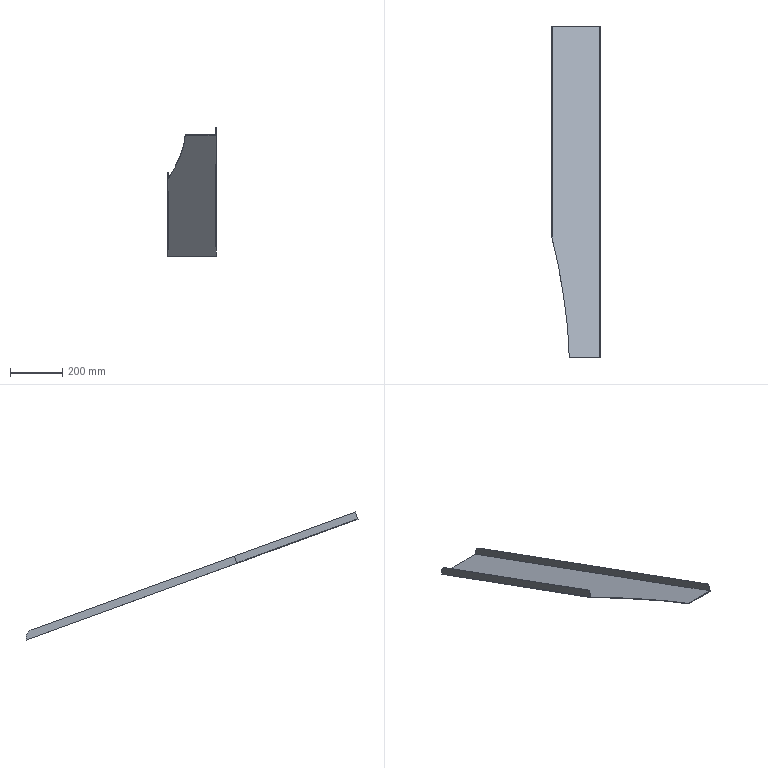Part | NX | features solid 2 | 1 solid | 15 faces | box 185.377 x 1270 x 489.666 mm | volume 582947 mm3 | plane 11 | spline 2 | cylinder 2 | commonest cylinder face diameters 60 x2
STEP:
#1=CARTESIAN_POINT('',(-110.,1180.,-569.375));
#2=VERTEX_POINT('',#1);
#3=CARTESIAN_POINT('',(-110.,-87.894,-107.899));
#4=VERTEX_POINT('',#3);
#5=CARTESIAN_POINT('',(-110.,-155.,-83.474));
#6=DIRECTION('',(0.,-0.9397,0.342));
#7=VECTOR('',#6,1000.);
#8=LINE('',#5,#7);
#9=EDGE_CURVE('',#2,#4,#8,.T.);
#10=ORIENTED_EDGE('',*,*,#9,.F.);
#11=CARTESIAN_POINT('',(-110.,1162.07,-530.923));
#12=VERTEX_POINT('',#11);
#13=CARTESIAN_POINT('',(-110.,1151.809,-559.114));
#14=DIRECTION('',(-1.,0.,0.));
#15=DIRECTION('',(0.,0.,1.));
#16=AXIS2_PLACEMENT_3D('',#13,#14,#15);
#17=CIRCLE('',#16,30.);
#18=EDGE_CURVE('',#2,#12,#17,.F.);
#19=ORIENTED_EDGE('',*,*,#18,.T.);
#20=CARTESIAN_POINT('',(-110.,-77.633,-79.708));
#21=VERTEX_POINT('',#20);
#22=CARTESIAN_POINT('',(-110.,1190.261,-541.184));
#23=DIRECTION('',(0.,-0.9397,0.342));
#24=VECTOR('',#23,1000.);
#25=LINE('',#22,#24);
#26=EDGE_CURVE('',#12,#21,#25,.T.);
#27=ORIENTED_EDGE('',*,*,#26,.T.);
#28=CARTESIAN_POINT('',(-110.,-87.21,-106.02));
#29=DIRECTION('',(0.,-0.342,-0.9397));
#30=VECTOR('',#29,1000.);
#31=LINE('',#28,#30);
#32=EDGE_CURVE('',#21,#4,#31,.T.);
#33=ORIENTED_EDGE('',*,*,#32,.T.);
#34=EDGE_LOOP('',(#10,#19,#27,#33));
#35=FACE_BOUND('',#34,.T.);
#36=CARTESIAN_POINT('',(-110.,-154.316,-81.595));
#37=DIRECTION('',(1.,0.,0.));
#38=DIRECTION('',(0.,0.,-1.));
#39=AXIS2_PLACEMENT_3D('',#36,#37,#38);
#40=PLANE('',#39);
#41=ADVANCED_FACE('',(#35),#40,.T.);
#42=CARTESIAN_POINT('',(-112.,1180.,-569.375));
#43=VERTEX_POINT('',#42);
#44=CARTESIAN_POINT('',(-112.,1180.,-567.246));
#45=VERTEX_POINT('',#44);
#46=CARTESIAN_POINT('',(-112.,1180.,-730.));
#47=DIRECTION('',(0.,0.,-1.));
#48=VECTOR('',#47,1000.);
#49=LINE('',#46,#48);
#50=EDGE_CURVE('',#43,#45,#49,.F.);
#51=ORIENTED_EDGE('',*,*,#50,.F.);
#52=CARTESIAN_POINT('',(-293.377,1180.,-569.375));
#53=VERTEX_POINT('',#52);
#54=CARTESIAN_POINT('',(-625.,1180.,-569.375));
#55=DIRECTION('',(-1.,0.,0.));
#56=VECTOR('',#55,1000.);
#57=LINE('',#54,#56);
#58=EDGE_CURVE('',#53,#43,#57,.F.);
#59=ORIENTED_EDGE('',*,*,#58,.F.);
#60=CARTESIAN_POINT('',(-293.377,1180.,-567.246));
#61=VERTEX_POINT('',#60);
#62=CARTESIAN_POINT('',(-293.377,1180.,-730.));
#63=DIRECTION('',(0.,0.,1.));
#64=VECTOR('',#63,1000.);
#65=LINE('',#62,#64);
#66=EDGE_CURVE('',#61,#53,#65,.F.);
#67=ORIENTED_EDGE('',*,*,#66,.F.);
#68=CARTESIAN_POINT('',(-625.,1180.,-567.246));
#69=DIRECTION('',(-1.,0.,0.));
#70=VECTOR('',#69,1000.);
#71=LINE('',#68,#70);
#72=EDGE_CURVE('',#61,#45,#71,.F.);
#73=ORIENTED_EDGE('',*,*,#72,.T.);
#74=EDGE_LOOP('',(#51,#59,#67,#73));
#75=FACE_BOUND('',#74,.T.);
#76=CARTESIAN_POINT('',(-625.,1180.,-730.));
#77=DIRECTION('',(0.,-1.,0.));
#78=DIRECTION('',(1.,0.,0.));
#79=AXIS2_PLACEMENT_3D('',#76,#77,#78);
#80=PLANE('',#79);
#81=ADVANCED_FACE('',(#75),#80,.F.);
#82=CARTESIAN_POINT('',(-295.377,1162.07,-530.923));
#83=VERTEX_POINT('',#82);
#84=CARTESIAN_POINT('',(-295.377,1180.,-569.375));
#85=VERTEX_POINT('',#84);
#86=CARTESIAN_POINT('',(-295.377,1151.809,-559.114));
#87=DIRECTION('',(1.,0.,0.));
#88=DIRECTION('',(0.,0.,-1.));
#89=AXIS2_PLACEMENT_3D('',#86,#87,#88);
#90=CIRCLE('',#89,30.);
#91=EDGE_CURVE('',#83,#85,#90,.F.);
#92=ORIENTED_EDGE('',*,*,#91,.T.);
#93=CARTESIAN_POINT('',(-295.377,375.,-276.379));
#94=VERTEX_POINT('',#93);
#95=CARTESIAN_POINT('',(-295.377,-155.,-83.474));
#96=DIRECTION('',(0.,-0.9397,0.342));
#97=VECTOR('',#96,1000.);
#98=LINE('',#95,#97);
#99=EDGE_CURVE('',#94,#85,#98,.F.);
#100=ORIENTED_EDGE('',*,*,#99,.F.);
#101=CARTESIAN_POINT('',(-295.377,375.684,-274.499));
#102=VERTEX_POINT('',#101);
#103=CARTESIAN_POINT('',(-295.377,375.,-276.379));
#104=CARTESIAN_POINT('',(-295.377,375.228,-275.752));
#105=CARTESIAN_POINT('',(-295.377,375.456,-275.126));
#106=CARTESIAN_POINT('',(-295.377,375.684,-274.499));
#107=B_SPLINE_CURVE_WITH_KNOTS('',3,(#103,#104,#105,#106),.UNSPECIFIED.,.F.,.F.,(4,4),(0.,1.),.UNSPECIFIED.);
#108=EDGE_CURVE('',#102,#94,#107,.F.);
#109=ORIENTED_EDGE('',*,*,#108,.F.);
#110=CARTESIAN_POINT('',(-295.377,385.261,-248.188));
#111=VERTEX_POINT('',#110);
#112=CARTESIAN_POINT('',(-295.377,375.,-276.379));
#113=DIRECTION('',(0.,0.342,0.9397));
#114=VECTOR('',#113,1000.);
#115=LINE('',#112,#114);
#116=EDGE_CURVE('',#102,#111,#115,.T.);
#117=ORIENTED_EDGE('',*,*,#116,.T.);
#118=CARTESIAN_POINT('',(-295.377,385.261,-248.188));
#119=DIRECTION('',(0.,0.9397,-0.342));
#120=VECTOR('',#119,1000.);
#121=LINE('',#118,#120);
#122=EDGE_CURVE('',#111,#83,#121,.T.);
#123=ORIENTED_EDGE('',*,*,#122,.T.);
#124=EDGE_LOOP('',(#92,#100,#109,#117,#123));
#125=FACE_BOUND('',#124,.T.);
#126=CARTESIAN_POINT('',(-295.377,-154.316,-81.595));
#127=DIRECTION('',(-1.,0.,0.));
#128=DIRECTION('',(0.,0.,1.));
#129=AXIS2_PLACEMENT_3D('',#126,#127,#128);
#130=PLANE('',#129);
#131=ADVANCED_FACE('',(#125),#130,.T.);
#132=CARTESIAN_POINT('',(-234.833,27.777,-150.));
#133=VERTEX_POINT('',#132);
#134=CARTESIAN_POINT('',(-295.377,375.,-276.379));
#135=CARTESIAN_POINT('',(-294.522,371.544,-275.121));
#136=CARTESIAN_POINT('',(-293.394,366.986,-273.462));
#137=CARTESIAN_POINT('',(-292.2,362.161,-271.706));
#138=CARTESIAN_POINT('',(-291.46,359.167,-270.616));
#139=CARTESIAN_POINT('',(-290.874,356.799,-269.754));
#140=CARTESIAN_POINT('',(-290.515,355.348,-269.226));
#141=CARTESIAN_POINT('',(-290.305,354.499,-268.917));
#142=CARTESIAN_POINT('',(-290.207,354.1,-268.772));
#143=CARTESIAN_POINT('',(-290.147,353.857,-268.683));
#144=CARTESIAN_POINT('',(-290.112,353.717,-268.632));
#145=CARTESIAN_POINT('',(-290.089,353.624,-268.598));
#146=CARTESIAN_POINT('',(-290.082,353.594,-268.588));
#147=CARTESIAN_POINT('',(-290.071,353.553,-268.573));
#148=CARTESIAN_POINT('',(-290.085,353.606,-268.592));
#149=CARTESIAN_POINT('',(-290.021,353.351,-268.499));
#150=CARTESIAN_POINT('',(-289.964,353.118,-268.414));
#151=CARTESIAN_POINT('',(-289.851,352.663,-268.249));
#152=CARTESIAN_POINT('',(-289.698,352.041,-268.022));
#153=CARTESIAN_POINT('',(-289.513,351.29,-267.749));
#154=CARTESIAN_POINT('',(-289.269,350.301,-267.389));
#155=CARTESIAN_POINT('',(-288.968,349.077,-266.943));
#156=CARTESIAN_POINT('',(-288.495,347.15,-266.242));
#157=CARTESIAN_POINT('',(-287.919,344.799,-265.386));
#158=CARTESIAN_POINT('',(-287.031,341.162,-264.063));
#159=CARTESIAN_POINT('',(-286.193,337.702,-262.803));
#160=CARTESIAN_POINT('',(-285.507,334.856,-261.767));
#161=CARTESIAN_POINT('',(-285.121,333.246,-261.182));
#162=CARTESIAN_POINT('',(-284.857,332.144,-260.78));
#163=CARTESIAN_POINT('',(-284.526,330.753,-260.274));
#164=CARTESIAN_POINT('',(-284.109,328.997,-259.635));
#165=CARTESIAN_POINT('',(-283.371,325.875,-258.499));
#166=CARTESIAN_POINT('',(-282.331,321.43,-256.881));
#167=CARTESIAN_POINT('',(-281.095,316.07,-254.93));
#168=CARTESIAN_POINT('',(-279.466,308.904,-252.322));
#169=CARTESIAN_POINT('',(-277.468,299.924,-249.053));
#170=CARTESIAN_POINT('',(-275.11,289.007,-245.08));
#171=CARTESIAN_POINT('',(-272.869,278.318,-241.189));
#172=CARTESIAN_POINT('',(-270.673,267.536,-237.265));
#173=CARTESIAN_POINT('',(-268.542,256.746,-233.338));
#174=CARTESIAN_POINT('',(-266.471,245.925,-229.399));
#175=CARTESIAN_POINT('',(-264.796,236.888,-226.11));
#176=CARTESIAN_POINT('',(-263.487,229.645,-223.474));
#177=CARTESIAN_POINT('',(-262.52,224.206,-221.494));
#178=CARTESIAN_POINT('',(-261.569,218.761,-219.512));
#179=CARTESIAN_POINT('',(-260.788,214.218,-217.859));
#180=CARTESIAN_POINT('',(-260.172,210.581,-216.535));
#181=CARTESIAN_POINT('',(-259.789,208.306,-215.707));
#182=CARTESIAN_POINT('',(-259.486,206.486,-215.044));
#183=CARTESIAN_POINT('',(-259.258,205.118,-214.547));
#184=CARTESIAN_POINT('',(-259.071,203.985,-214.134));
#185=CARTESIAN_POINT('',(-258.938,203.177,-213.84));
#186=CARTESIAN_POINT('',(-258.866,202.739,-213.681));
#187=CARTESIAN_POINT('',(-258.801,202.344,-213.537));
#188=CARTESIAN_POINT('',(-258.777,202.201,-213.485));
#189=CARTESIAN_POINT('',(-258.731,201.919,-213.382));
#190=CARTESIAN_POINT('',(-258.655,201.457,-213.214));
#191=CARTESIAN_POINT('',(-258.541,200.755,-212.959));
#192=CARTESIAN_POINT('',(-258.399,199.884,-212.642));
#193=CARTESIAN_POINT('',(-258.203,198.672,-212.2));
#194=CARTESIAN_POINT('',(-257.944,197.067,-211.616));
#195=CARTESIAN_POINT('',(-257.5,194.306,-210.612));
#196=CARTESIAN_POINT('',(-256.893,190.493,-209.224));
#197=CARTESIAN_POINT('',(-256.077,185.337,-207.347));
#198=CARTESIAN_POINT('',(-255.175,179.603,-205.26));
#199=CARTESIAN_POINT('',(-254.351,174.341,-203.345));
#200=CARTESIAN_POINT('',(-253.65,169.842,-201.707));
#201=CARTESIAN_POINT('',(-253.101,166.32,-200.425));
#202=CARTESIAN_POINT('',(-252.628,163.276,-199.317));
#203=CARTESIAN_POINT('',(-252.284,161.059,-198.51));
#204=CARTESIAN_POINT('',(-252.09,159.809,-198.056));
#205=CARTESIAN_POINT('',(-251.928,158.763,-197.675));
#206=CARTESIAN_POINT('',(-251.823,158.091,-197.43));
#207=CARTESIAN_POINT('',(-251.665,157.071,-197.059));
#208=CARTESIAN_POINT('',(-251.4,155.363,-196.437));
#209=CARTESIAN_POINT('',(-251.023,152.936,-195.554));
#210=CARTESIAN_POINT('',(-250.584,150.108,-194.525));
#211=CARTESIAN_POINT('',(-250.155,147.348,-193.52));
#212=CARTESIAN_POINT('',(-249.736,144.661,-192.542));
#213=CARTESIAN_POINT('',(-249.396,142.48,-191.748));
#214=CARTESIAN_POINT('',(-249.13,140.771,-191.126));
#215=CARTESIAN_POINT('',(-248.933,139.509,-190.667));
#216=CARTESIAN_POINT('',(-248.77,138.465,-190.287));
#217=CARTESIAN_POINT('',(-248.659,137.756,-190.029));
#218=CARTESIAN_POINT('',(-248.593,137.331,-189.874));
#219=CARTESIAN_POINT('',(-248.553,137.076,-189.781));
#220=CARTESIAN_POINT('',(-248.476,136.582,-189.602));
#221=CARTESIAN_POINT('',(-248.387,136.012,-189.394));
#222=CARTESIAN_POINT('',(-248.227,134.988,-189.021));
#223=CARTESIAN_POINT('',(-248.007,133.577,-188.508));
#224=CARTESIAN_POINT('',(-247.75,131.927,-187.907));
#225=CARTESIAN_POINT('',(-247.419,129.799,-187.133));
#226=CARTESIAN_POINT('',(-247.027,127.269,-186.212));
#227=CARTESIAN_POINT('',(-246.445,123.497,-184.839));
#228=CARTESIAN_POINT('',(-245.933,120.148,-183.62));
#229=CARTESIAN_POINT('',(-245.542,117.565,-182.68));
#230=CARTESIAN_POINT('',(-245.364,116.387,-182.251));
#231=CARTESIAN_POINT('',(-245.262,115.705,-182.003));
#232=CARTESIAN_POINT('',(-245.202,115.303,-181.857));
#233=CARTESIAN_POINT('',(-245.089,114.544,-181.58));
#234=CARTESIAN_POINT('',(-244.957,113.656,-181.257));
#235=CARTESIAN_POINT('',(-244.787,112.504,-180.838));
#236=CARTESIAN_POINT('',(-244.587,111.14,-180.341));
#237=CARTESIAN_POINT('',(-244.32,109.315,-179.677));
#238=CARTESIAN_POINT('',(-243.991,107.035,-178.848));
#239=CARTESIAN_POINT('',(-243.471,103.388,-177.52));
#240=CARTESIAN_POINT('',(-242.834,98.829,-175.861));
#241=CARTESIAN_POINT('',(-242.091,93.359,-173.87));
#242=CARTESIAN_POINT('',(-241.369,87.889,-171.879));
#243=CARTESIAN_POINT('',(-240.435,80.598,-169.225));
#244=CARTESIAN_POINT('',(-238.874,67.841,-164.582));
#245=CARTESIAN_POINT('',(-236.855,49.624,-157.951));
#246=CARTESIAN_POINT('',(-235.465,35.058,-152.65));
#247=CARTESIAN_POINT('',(-234.826,27.777,-150.));
#248=B_SPLINE_CURVE_WITH_KNOTS('',3,(#134,#135,#136,#137,#138,#139,#140,#141,#142,#143,#144,#145,#146,#147,#148,#149,#150,#151,#152,#153,#154,#155,#156,#157,#158,#159,#160,#161,#162,#163,#164,#165,#166,#167,#168,#169,#170,#171,#172,#173,#174,#175,#176,#177,#178,#179,#180,#181,#182,#183,#184,#185,#186,#187,#188,#189,#190,#191,#192,#193,#194,#195,#196,#197,#198,#199,#200,#201,#202,#203,#204,#205,#206,#207,#208,#209,#210,#211,#212,#213,#214,#215,#216,#217,#218,#219,#220,#221,#222,#223,#224,#225,#226,#227,#228,#229,#230,#231,#232,#233,#234,#235,#236,#237,#238,#239,#240,#241,#242,#243,#244,#245,#246,#247),.UNSPECIFIED.,.F.,.F.,(4,1,1,1,1,1,1,1,1,1,1,1,1,1,1,1,1,1,1,1,1,1,1,1,1,1,1,1,1,1,1,1,1,1,1,1,1,1,1,1,1,1,1,1,1,1,1,1,1,1,1,1,1,1,1,1,1,1,1,1,1,1,1,1,1,1,1,1,1,1,1,1,1,1,1,1,1,1,1,1,1,1,1,1,1,1,1,1,1,1,1,1,1,1,1,1,1,1,1,1,1,1,1,1,1,1,1,1,1,1,1,4),(0.,0.01562,0.02344,0.03125,0.03906,0.04688,0.05078,0.05469,0.05664,0.05859,0.06055,0.06152,0.06201,0.0625,0.06299,0.06348,0.06445,0.06641,0.06836,0.07031,0.07422,0.07812,0.08594,0.09375,0.1094,0.1172,0.1211,0.125,0.1289,0.1328,0.1406,0.1562,0.1719,0.1875,0.2188,0.25,0.2812,0.3125,0.3438,0.375,0.4062,0.4219,0.4375,0.4531,0.4688,0.4766,0.4844,0.4883,0.4922,0.4961,0.498,0.499,0.5,0.501,0.502,0.5039,0.5078,0.5117,0.5156,0.5234,0.5312,0.5469,0.5625,0.5781,0.5938,0.6016,0.6094,0.6172,0.6211,0.623,0.625,0.627,0.6289,0.6328,0.6406,0.6484,0.6562,0.6641,0.6719,0.6758,0.6797,0.6836,0.6855,0.6865,0.6875,0.6885,0.6895,0.6914,0.6953,0.6992,0.7031,0.7109,0.7188,0.7344,0.7422,0.7461,0.748,0.75,0.752,0.7539,0.7578,0.7617,0.7656,0.7734,0.7812,0.7969,0.8125,0.8281,0.8438,0.875,0.9375,1.),.UNSPECIFIED.);
#249=EDGE_CURVE('',#94,#133,#248,.T.);
#250=ORIENTED_EDGE('',*,*,#249,.T.);
#251=CARTESIAN_POINT('',(-234.833,28.461,-148.121));
#252=VERTEX_POINT('',#251);
#253=CARTESIAN_POINT('',(-234.826,27.778,-150.));
#254=CARTESIAN_POINT('',(-234.826,28.006,-149.374));
#255=CARTESIAN_POINT('',(-234.826,28.234,-148.747));
#256=CARTESIAN_POINT('',(-234.826,28.462,-148.121));
#257=B_SPLINE_CURVE_WITH_KNOTS('',3,(#253,#254,#255,#256),.UNSPECIFIED.,.F.,.F.,(4,4),(0.,1.),.UNSPECIFIED.);
#258=EDGE_CURVE('',#252,#133,#257,.F.);
#259=ORIENTED_EDGE('',*,*,#258,.F.);
#260=CARTESIAN_POINT('',(-295.377,375.684,-274.499));
#261=CARTESIAN_POINT('',(-294.522,372.228,-273.241));
#262=CARTESIAN_POINT('',(-293.394,367.67,-271.583));
#263=CARTESIAN_POINT('',(-292.2,362.845,-269.826));
#264=CARTESIAN_POINT('',(-291.46,359.851,-268.737));
#265=CARTESIAN_POINT('',(-290.874,357.483,-267.875));
#266=CARTESIAN_POINT('',(-290.515,356.032,-267.346));
#267=CARTESIAN_POINT('',(-290.305,355.183,-267.038));
#268=CARTESIAN_POINT('',(-290.207,354.784,-266.892));
#269=CARTESIAN_POINT('',(-290.147,354.541,-266.804));
#270=CARTESIAN_POINT('',(-290.112,354.401,-266.753));
#271=CARTESIAN_POINT('',(-290.089,354.308,-266.719));
#272=CARTESIAN_POINT('',(-290.082,354.278,-266.708));
#273=CARTESIAN_POINT('',(-290.071,354.237,-266.693));
#274=CARTESIAN_POINT('',(-290.085,354.29,-266.713));
#275=CARTESIAN_POINT('',(-290.021,354.035,-266.62));
#276=CARTESIAN_POINT('',(-289.964,353.802,-266.535));
#277=CARTESIAN_POINT('',(-289.851,353.347,-266.369));
#278=CARTESIAN_POINT('',(-289.698,352.725,-266.143));
#279=CARTESIAN_POINT('',(-289.513,351.975,-265.87));
#280=CARTESIAN_POINT('',(-289.269,350.985,-265.51));
#281=CARTESIAN_POINT('',(-288.968,349.761,-265.064));
#282=CARTESIAN_POINT('',(-288.495,347.834,-264.363));
#283=CARTESIAN_POINT('',(-287.919,345.483,-263.507));
#284=CARTESIAN_POINT('',(-287.031,341.846,-262.183));
#285=CARTESIAN_POINT('',(-286.193,338.386,-260.924));
#286=CARTESIAN_POINT('',(-285.507,335.54,-259.888));
#287=CARTESIAN_POINT('',(-285.121,333.93,-259.302));
#288=CARTESIAN_POINT('',(-284.857,332.828,-258.901));
#289=CARTESIAN_POINT('',(-284.526,331.437,-258.395));
#290=CARTESIAN_POINT('',(-284.109,329.682,-257.756));
#291=CARTESIAN_POINT('',(-283.371,326.559,-256.619));
#292=CARTESIAN_POINT('',(-282.331,322.114,-255.001));
#293=CARTESIAN_POINT('',(-281.095,316.754,-253.05));
#294=CARTESIAN_POINT('',(-279.466,309.588,-250.442));
#295=CARTESIAN_POINT('',(-277.468,300.608,-247.174));
#296=CARTESIAN_POINT('',(-275.11,289.691,-243.201));
#297=CARTESIAN_POINT('',(-272.869,279.002,-239.31));
#298=CARTESIAN_POINT('',(-270.673,268.22,-235.386));
#299=CARTESIAN_POINT('',(-268.542,257.43,-231.458));
#300=CARTESIAN_POINT('',(-266.471,246.609,-227.52));
#301=CARTESIAN_POINT('',(-264.796,237.572,-224.231));
#302=CARTESIAN_POINT('',(-263.487,230.329,-221.594));
#303=CARTESIAN_POINT('',(-262.52,224.89,-219.615));
#304=CARTESIAN_POINT('',(-261.569,219.445,-217.633));
#305=CARTESIAN_POINT('',(-260.788,214.902,-215.979));
#306=CARTESIAN_POINT('',(-260.172,211.265,-214.656));
#307=CARTESIAN_POINT('',(-259.789,208.99,-213.827));
#308=CARTESIAN_POINT('',(-259.486,207.17,-213.165));
#309=CARTESIAN_POINT('',(-259.258,205.802,-212.667));
#310=CARTESIAN_POINT('',(-259.071,204.669,-212.255));
#311=CARTESIAN_POINT('',(-258.938,203.861,-211.961));
#312=CARTESIAN_POINT('',(-258.866,203.423,-211.801));
#313=CARTESIAN_POINT('',(-258.801,203.028,-211.658));
#314=CARTESIAN_POINT('',(-258.777,202.885,-211.606));
#315=CARTESIAN_POINT('',(-258.731,202.603,-211.503));
#316=CARTESIAN_POINT('',(-258.655,202.141,-211.335));
#317=CARTESIAN_POINT('',(-258.541,201.439,-211.079));
#318=CARTESIAN_POINT('',(-258.399,200.568,-210.762));
#319=CARTESIAN_POINT('',(-258.203,199.356,-210.321));
#320=CARTESIAN_POINT('',(-257.944,197.751,-209.737));
#321=CARTESIAN_POINT('',(-257.5,194.99,-208.732));
#322=CARTESIAN_POINT('',(-256.893,191.177,-207.344));
#323=CARTESIAN_POINT('',(-256.077,186.022,-205.468));
#324=CARTESIAN_POINT('',(-255.175,180.287,-203.381));
#325=CARTESIAN_POINT('',(-254.351,175.025,-201.465));
#326=CARTESIAN_POINT('',(-253.65,170.526,-199.828));
#327=CARTESIAN_POINT('',(-253.101,167.004,-198.546));
#328=CARTESIAN_POINT('',(-252.628,163.96,-197.438));
#329=CARTESIAN_POINT('',(-252.284,161.743,-196.631));
#330=CARTESIAN_POINT('',(-252.09,160.493,-196.176));
#331=CARTESIAN_POINT('',(-251.928,159.447,-195.795));
#332=CARTESIAN_POINT('',(-251.823,158.775,-195.551));
#333=CARTESIAN_POINT('',(-251.665,157.755,-195.18));
#334=CARTESIAN_POINT('',(-251.4,156.047,-194.558));
#335=CARTESIAN_POINT('',(-251.023,153.62,-193.675));
#336=CARTESIAN_POINT('',(-250.584,150.793,-192.645));
#337=CARTESIAN_POINT('',(-250.155,148.033,-191.641));
#338=CARTESIAN_POINT('',(-249.736,145.345,-190.663));
#339=CARTESIAN_POINT('',(-249.396,143.164,-189.869));
#340=CARTESIAN_POINT('',(-249.13,141.455,-189.247));
#341=CARTESIAN_POINT('',(-248.933,140.193,-188.788));
#342=CARTESIAN_POINT('',(-248.77,139.149,-188.407));
#343=CARTESIAN_POINT('',(-248.659,138.44,-188.15));
#344=CARTESIAN_POINT('',(-248.593,138.015,-187.995));
#345=CARTESIAN_POINT('',(-248.553,137.76,-187.902));
#346=CARTESIAN_POINT('',(-248.476,137.266,-187.722));
#347=CARTESIAN_POINT('',(-248.387,136.697,-187.515));
#348=CARTESIAN_POINT('',(-248.227,135.672,-187.142));
#349=CARTESIAN_POINT('',(-248.007,134.261,-186.628));
#350=CARTESIAN_POINT('',(-247.75,132.611,-186.028));
#351=CARTESIAN_POINT('',(-247.419,130.483,-185.253));
#352=CARTESIAN_POINT('',(-247.027,127.953,-184.332));
#353=CARTESIAN_POINT('',(-246.445,124.181,-182.96));
#354=CARTESIAN_POINT('',(-245.933,120.832,-181.741));
#355=CARTESIAN_POINT('',(-245.542,118.249,-180.801));
#356=CARTESIAN_POINT('',(-245.364,117.071,-180.372));
#357=CARTESIAN_POINT('',(-245.262,116.389,-180.123));
#358=CARTESIAN_POINT('',(-245.202,115.987,-179.977));
#359=CARTESIAN_POINT('',(-245.089,115.228,-179.701));
#360=CARTESIAN_POINT('',(-244.957,114.34,-179.378));
#361=CARTESIAN_POINT('',(-244.787,113.188,-178.959));
#362=CARTESIAN_POINT('',(-244.587,111.824,-178.462));
#363=CARTESIAN_POINT('',(-244.32,109.999,-177.798));
#364=CARTESIAN_POINT('',(-243.991,107.719,-176.968));
#365=CARTESIAN_POINT('',(-243.471,104.072,-175.64));
#366=CARTESIAN_POINT('',(-242.834,99.513,-173.981));
#367=CARTESIAN_POINT('',(-242.091,94.043,-171.99));
#368=CARTESIAN_POINT('',(-241.369,88.573,-170.));
#369=CARTESIAN_POINT('',(-240.435,81.282,-167.346));
#370=CARTESIAN_POINT('',(-238.874,68.525,-162.702));
#371=CARTESIAN_POINT('',(-236.855,50.308,-156.072));
#372=CARTESIAN_POINT('',(-235.465,35.742,-150.771));
#373=CARTESIAN_POINT('',(-234.826,28.462,-148.121));
#374=B_SPLINE_CURVE_WITH_KNOTS('',3,(#260,#261,#262,#263,#264,#265,#266,#267,#268,#269,#270,#271,#272,#273,#274,#275,#276,#277,#278,#279,#280,#281,#282,#283,#284,#285,#286,#287,#288,#289,#290,#291,#292,#293,#294,#295,#296,#297,#298,#299,#300,#301,#302,#303,#304,#305,#306,#307,#308,#309,#310,#311,#312,#313,#314,#315,#316,#317,#318,#319,#320,#321,#322,#323,#324,#325,#326,#327,#328,#329,#330,#331,#332,#333,#334,#335,#336,#337,#338,#339,#340,#341,#342,#343,#344,#345,#346,#347,#348,#349,#350,#351,#352,#353,#354,#355,#356,#357,#358,#359,#360,#361,#362,#363,#364,#365,#366,#367,#368,#369,#370,#371,#372,#373),.UNSPECIFIED.,.F.,.F.,(4,1,1,1,1,1,1,1,1,1,1,1,1,1,1,1,1,1,1,1,1,1,1,1,1,1,1,1,1,1,1,1,1,1,1,1,1,1,1,1,1,1,1,1,1,1,1,1,1,1,1,1,1,1,1,1,1,1,1,1,1,1,1,1,1,1,1,1,1,1,1,1,1,1,1,1,1,1,1,1,1,1,1,1,1,1,1,1,1,1,1,1,1,1,1,1,1,1,1,1,1,1,1,1,1,1,1,1,1,1,1,4),(0.,0.01562,0.02344,0.03125,0.03906,0.04688,0.05078,0.05469,0.05664,0.05859,0.06055,0.06152,0.06201,0.0625,0.06299,0.06348,0.06445,0.06641,0.06836,0.07031,0.07422,0.07812,0.08594,0.09375,0.1094,0.1172,0.1211,0.125,0.1289,0.1328,0.1406,0.1562,0.1719,0.1875,0.2188,0.25,0.2812,0.3125,0.3438,0.375,0.4062,0.4219,0.4375,0.4531,0.4688,0.4766,0.4844,0.4883,0.4922,0.4961,0.498,0.499,0.5,0.501,0.502,0.5039,0.5078,0.5117,0.5156,0.5234,0.5312,0.5469,0.5625,0.5781,0.5938,0.6016,0.6094,0.6172,0.6211,0.623,0.625,0.627,0.6289,0.6328,0.6406,0.6484,0.6562,0.6641,0.6719,0.6758,0.6797,0.6836,0.6855,0.6865,0.6875,0.6885,0.6895,0.6914,0.6953,0.6992,0.7031,0.7109,0.7188,0.7344,0.7422,0.7461,0.748,0.75,0.752,0.7539,0.7578,0.7617,0.7656,0.7734,0.7812,0.7969,0.8125,0.8281,0.8438,0.875,0.9375,1.),.UNSPECIFIED.);
#375=EDGE_CURVE('',#102,#252,#374,.T.);
#376=ORIENTED_EDGE('',*,*,#375,.F.);
#377=ORIENTED_EDGE('',*,*,#108,.T.);
#378=EDGE_LOOP('',(#250,#259,#376,#377));
#379=FACE_BOUND('',#378,.T.);
#380=CARTESIAN_POINT('',(-295.377,375.684,-274.499));
#381=CARTESIAN_POINT('',(-295.377,375.,-276.379));
#382=CARTESIAN_POINT('',(-294.522,372.228,-273.241));
#383=CARTESIAN_POINT('',(-294.522,371.544,-275.121));
#384=CARTESIAN_POINT('',(-293.394,367.67,-271.583));
#385=CARTESIAN_POINT('',(-293.394,366.986,-273.462));
#386=CARTESIAN_POINT('',(-292.2,362.845,-269.826));
#387=CARTESIAN_POINT('',(-292.2,362.161,-271.706));
#388=CARTESIAN_POINT('',(-291.46,359.851,-268.737));
#389=CARTESIAN_POINT('',(-291.46,359.167,-270.616));
#390=CARTESIAN_POINT('',(-290.874,357.483,-267.875));
#391=CARTESIAN_POINT('',(-290.874,356.799,-269.754));
#392=CARTESIAN_POINT('',(-290.515,356.032,-267.346));
#393=CARTESIAN_POINT('',(-290.515,355.348,-269.226));
#394=CARTESIAN_POINT('',(-290.305,355.183,-267.038));
#395=CARTESIAN_POINT('',(-290.305,354.499,-268.917));
#396=CARTESIAN_POINT('',(-290.207,354.784,-266.892));
#397=CARTESIAN_POINT('',(-290.207,354.1,-268.772));
#398=CARTESIAN_POINT('',(-290.147,354.541,-266.804));
#399=CARTESIAN_POINT('',(-290.147,353.857,-268.683));
#400=CARTESIAN_POINT('',(-290.112,354.401,-266.753));
#401=CARTESIAN_POINT('',(-290.112,353.717,-268.632));
#402=CARTESIAN_POINT('',(-290.089,354.308,-266.719));
#403=CARTESIAN_POINT('',(-290.089,353.624,-268.598));
#404=CARTESIAN_POINT('',(-290.082,354.278,-266.708));
#405=CARTESIAN_POINT('',(-290.082,353.594,-268.588));
#406=CARTESIAN_POINT('',(-290.071,354.237,-266.693));
#407=CARTESIAN_POINT('',(-290.071,353.553,-268.573));
#408=CARTESIAN_POINT('',(-290.085,354.29,-266.713));
#409=CARTESIAN_POINT('',(-290.085,353.606,-268.592));
#410=CARTESIAN_POINT('',(-290.021,354.035,-266.62));
#411=CARTESIAN_POINT('',(-290.021,353.351,-268.499));
#412=CARTESIAN_POINT('',(-289.964,353.802,-266.535));
#413=CARTESIAN_POINT('',(-289.964,353.118,-268.414));
#414=CARTESIAN_POINT('',(-289.851,353.347,-266.369));
#415=CARTESIAN_POINT('',(-289.851,352.663,-268.249));
#416=CARTESIAN_POINT('',(-289.698,352.725,-266.143));
#417=CARTESIAN_POINT('',(-289.698,352.041,-268.022));
#418=CARTESIAN_POINT('',(-289.513,351.975,-265.87));
#419=CARTESIAN_POINT('',(-289.513,351.29,-267.749));
#420=CARTESIAN_POINT('',(-289.269,350.985,-265.51));
#421=CARTESIAN_POINT('',(-289.269,350.301,-267.389));
#422=CARTESIAN_POINT('',(-288.968,349.761,-265.064));
#423=CARTESIAN_POINT('',(-288.968,349.077,-266.943));
#424=CARTESIAN_POINT('',(-288.495,347.834,-264.363));
#425=CARTESIAN_POINT('',(-288.495,347.15,-266.242));
#426=CARTESIAN_POINT('',(-287.919,345.483,-263.507));
#427=CARTESIAN_POINT('',(-287.919,344.799,-265.386));
#428=CARTESIAN_POINT('',(-287.031,341.846,-262.183));
#429=CARTESIAN_POINT('',(-287.031,341.162,-264.063));
#430=CARTESIAN_POINT('',(-286.193,338.386,-260.924));
#431=CARTESIAN_POINT('',(-286.193,337.702,-262.803));
#432=CARTESIAN_POINT('',(-285.507,335.54,-259.888));
#433=CARTESIAN_POINT('',(-285.507,334.856,-261.767));
#434=CARTESIAN_POINT('',(-285.121,333.93,-259.302));
#435=CARTESIAN_POINT('',(-285.121,333.246,-261.182));
#436=CARTESIAN_POINT('',(-284.857,332.828,-258.901));
#437=CARTESIAN_POINT('',(-284.857,332.144,-260.78));
#438=CARTESIAN_POINT('',(-284.526,331.437,-258.395));
#439=CARTESIAN_POINT('',(-284.526,330.753,-260.274));
#440=CARTESIAN_POINT('',(-284.109,329.682,-257.756));
#441=CARTESIAN_POINT('',(-284.109,328.997,-259.635));
#442=CARTESIAN_POINT('',(-283.371,326.559,-256.619));
#443=CARTESIAN_POINT('',(-283.371,325.875,-258.499));
#444=CARTESIAN_POINT('',(-282.331,322.114,-255.001));
#445=CARTESIAN_POINT('',(-282.331,321.43,-256.881));
#446=CARTESIAN_POINT('',(-281.095,316.754,-253.05));
#447=CARTESIAN_POINT('',(-281.095,316.07,-254.93));
#448=CARTESIAN_POINT('',(-279.466,309.588,-250.442));
#449=CARTESIAN_POINT('',(-279.466,308.904,-252.322));
#450=CARTESIAN_POINT('',(-277.468,300.608,-247.174));
#451=CARTESIAN_POINT('',(-277.468,299.924,-249.053));
#452=CARTESIAN_POINT('',(-275.11,289.691,-243.201));
#453=CARTESIAN_POINT('',(-275.11,289.007,-245.08));
#454=CARTESIAN_POINT('',(-272.869,279.002,-239.31));
#455=CARTESIAN_POINT('',(-272.869,278.318,-241.189));
#456=CARTESIAN_POINT('',(-270.673,268.22,-235.386));
#457=CARTESIAN_POINT('',(-270.673,267.536,-237.265));
#458=CARTESIAN_POINT('',(-268.542,257.43,-231.458));
#459=CARTESIAN_POINT('',(-268.542,256.746,-233.338));
#460=CARTESIAN_POINT('',(-266.471,246.609,-227.52));
#461=CARTESIAN_POINT('',(-266.471,245.925,-229.399));
#462=CARTESIAN_POINT('',(-264.796,237.572,-224.231));
#463=CARTESIAN_POINT('',(-264.796,236.888,-226.11));
#464=CARTESIAN_POINT('',(-263.487,230.329,-221.594));
#465=CARTESIAN_POINT('',(-263.487,229.645,-223.474));
#466=CARTESIAN_POINT('',(-262.52,224.89,-219.615));
#467=CARTESIAN_POINT('',(-262.52,224.206,-221.494));
#468=CARTESIAN_POINT('',(-261.569,219.445,-217.633));
#469=CARTESIAN_POINT('',(-261.569,218.761,-219.512));
#470=CARTESIAN_POINT('',(-260.788,214.902,-215.979));
#471=CARTESIAN_POINT('',(-260.788,214.218,-217.859));
#472=CARTESIAN_POINT('',(-260.172,211.265,-214.656));
#473=CARTESIAN_POINT('',(-260.172,210.581,-216.535));
#474=CARTESIAN_POINT('',(-259.789,208.99,-213.827));
#475=CARTESIAN_POINT('',(-259.789,208.306,-215.707));
#476=CARTESIAN_POINT('',(-259.486,207.17,-213.165));
#477=CARTESIAN_POINT('',(-259.486,206.486,-215.044));
#478=CARTESIAN_POINT('',(-259.258,205.802,-212.667));
#479=CARTESIAN_POINT('',(-259.258,205.118,-214.547));
#480=CARTESIAN_POINT('',(-259.071,204.669,-212.255));
#481=CARTESIAN_POINT('',(-259.071,203.985,-214.134));
#482=CARTESIAN_POINT('',(-258.938,203.861,-211.961));
#483=CARTESIAN_POINT('',(-258.938,203.177,-213.84));
#484=CARTESIAN_POINT('',(-258.866,203.423,-211.801));
#485=CARTESIAN_POINT('',(-258.866,202.739,-213.681));
#486=CARTESIAN_POINT('',(-258.801,203.028,-211.658));
#487=CARTESIAN_POINT('',(-258.801,202.344,-213.537));
#488=CARTESIAN_POINT('',(-258.777,202.885,-211.606));
#489=CARTESIAN_POINT('',(-258.777,202.201,-213.485));
#490=CARTESIAN_POINT('',(-258.731,202.603,-211.503));
#491=CARTESIAN_POINT('',(-258.731,201.919,-213.382));
#492=CARTESIAN_POINT('',(-258.655,202.141,-211.335));
#493=CARTESIAN_POINT('',(-258.655,201.457,-213.214));
#494=CARTESIAN_POINT('',(-258.541,201.439,-211.079));
#495=CARTESIAN_POINT('',(-258.541,200.755,-212.959));
#496=CARTESIAN_POINT('',(-258.399,200.568,-210.762));
#497=CARTESIAN_POINT('',(-258.399,199.884,-212.642));
#498=CARTESIAN_POINT('',(-258.203,199.356,-210.321));
#499=CARTESIAN_POINT('',(-258.203,198.672,-212.2));
#500=CARTESIAN_POINT('',(-257.944,197.751,-209.737));
#501=CARTESIAN_POINT('',(-257.944,197.067,-211.616));
#502=CARTESIAN_POINT('',(-257.5,194.99,-208.732));
#503=CARTESIAN_POINT('',(-257.5,194.306,-210.612));
#504=CARTESIAN_POINT('',(-256.893,191.177,-207.344));
#505=CARTESIAN_POINT('',(-256.893,190.493,-209.224));
#506=CARTESIAN_POINT('',(-256.077,186.022,-205.468));
#507=CARTESIAN_POINT('',(-256.077,185.337,-207.347));
#508=CARTESIAN_POINT('',(-255.175,180.287,-203.381));
#509=CARTESIAN_POINT('',(-255.175,179.603,-205.26));
#510=CARTESIAN_POINT('',(-254.351,175.025,-201.465));
#511=CARTESIAN_POINT('',(-254.351,174.341,-203.345));
#512=CARTESIAN_POINT('',(-253.65,170.526,-199.828));
#513=CARTESIAN_POINT('',(-253.65,169.842,-201.707));
#514=CARTESIAN_POINT('',(-253.101,167.004,-198.546));
#515=CARTESIAN_POINT('',(-253.101,166.32,-200.425));
#516=CARTESIAN_POINT('',(-252.628,163.96,-197.438));
#517=CARTESIAN_POINT('',(-252.628,163.276,-199.317));
#518=CARTESIAN_POINT('',(-252.284,161.743,-196.631));
#519=CARTESIAN_POINT('',(-252.284,161.059,-198.51));
#520=CARTESIAN_POINT('',(-252.09,160.493,-196.176));
#521=CARTESIAN_POINT('',(-252.09,159.809,-198.056));
#522=CARTESIAN_POINT('',(-251.928,159.447,-195.795));
#523=CARTESIAN_POINT('',(-251.928,158.763,-197.675));
#524=CARTESIAN_POINT('',(-251.823,158.775,-195.551));
#525=CARTESIAN_POINT('',(-251.823,158.091,-197.43));
#526=CARTESIAN_POINT('',(-251.665,157.755,-195.18));
#527=CARTESIAN_POINT('',(-251.665,157.071,-197.059));
#528=CARTESIAN_POINT('',(-251.4,156.047,-194.558));
#529=CARTESIAN_POINT('',(-251.4,155.363,-196.437));
#530=CARTESIAN_POINT('',(-251.023,153.62,-193.675));
#531=CARTESIAN_POINT('',(-251.023,152.936,-195.554));
#532=CARTESIAN_POINT('',(-250.584,150.793,-192.645));
#533=CARTESIAN_POINT('',(-250.584,150.108,-194.525));
#534=CARTESIAN_POINT('',(-250.155,148.033,-191.641));
#535=CARTESIAN_POINT('',(-250.155,147.348,-193.52));
#536=CARTESIAN_POINT('',(-249.736,145.345,-190.663));
#537=CARTESIAN_POINT('',(-249.736,144.661,-192.542));
#538=CARTESIAN_POINT('',(-249.396,143.164,-189.869));
#539=CARTESIAN_POINT('',(-249.396,142.48,-191.748));
#540=CARTESIAN_POINT('',(-249.13,141.455,-189.247));
#541=CARTESIAN_POINT('',(-249.13,140.771,-191.126));
#542=CARTESIAN_POINT('',(-248.933,140.193,-188.788));
#543=CARTESIAN_POINT('',(-248.933,139.509,-190.667));
#544=CARTESIAN_POINT('',(-248.77,139.149,-188.407));
#545=CARTESIAN_POINT('',(-248.77,138.465,-190.287));
#546=CARTESIAN_POINT('',(-248.659,138.44,-188.15));
#547=CARTESIAN_POINT('',(-248.659,137.756,-190.029));
#548=CARTESIAN_POINT('',(-248.593,138.015,-187.995));
#549=CARTESIAN_POINT('',(-248.593,137.331,-189.874));
#550=CARTESIAN_POINT('',(-248.553,137.76,-187.902));
#551=CARTESIAN_POINT('',(-248.553,137.076,-189.781));
#552=CARTESIAN_POINT('',(-248.476,137.266,-187.722));
#553=CARTESIAN_POINT('',(-248.476,136.582,-189.602));
#554=CARTESIAN_POINT('',(-248.387,136.697,-187.515));
#555=CARTESIAN_POINT('',(-248.387,136.012,-189.394));
#556=CARTESIAN_POINT('',(-248.227,135.672,-187.142));
#557=CARTESIAN_POINT('',(-248.227,134.988,-189.021));
#558=CARTESIAN_POINT('',(-248.007,134.261,-186.628));
#559=CARTESIAN_POINT('',(-248.007,133.577,-188.508));
#560=CARTESIAN_POINT('',(-247.75,132.611,-186.028));
#561=CARTESIAN_POINT('',(-247.75,131.927,-187.907));
#562=CARTESIAN_POINT('',(-247.419,130.483,-185.253));
#563=CARTESIAN_POINT('',(-247.419,129.799,-187.133));
#564=CARTESIAN_POINT('',(-247.027,127.953,-184.332));
#565=CARTESIAN_POINT('',(-247.027,127.269,-186.212));
#566=CARTESIAN_POINT('',(-246.445,124.181,-182.96));
#567=CARTESIAN_POINT('',(-246.445,123.497,-184.839));
#568=CARTESIAN_POINT('',(-245.933,120.832,-181.741));
#569=CARTESIAN_POINT('',(-245.933,120.148,-183.62));
#570=CARTESIAN_POINT('',(-245.542,118.249,-180.801));
#571=CARTESIAN_POINT('',(-245.542,117.565,-182.68));
#572=CARTESIAN_POINT('',(-245.364,117.071,-180.372));
#573=CARTESIAN_POINT('',(-245.364,116.387,-182.251));
#574=CARTESIAN_POINT('',(-245.262,116.389,-180.123));
#575=CARTESIAN_POINT('',(-245.262,115.705,-182.003));
#576=CARTESIAN_POINT('',(-245.202,115.987,-179.977));
#577=CARTESIAN_POINT('',(-245.202,115.303,-181.857));
#578=CARTESIAN_POINT('',(-245.089,115.228,-179.701));
#579=CARTESIAN_POINT('',(-245.089,114.544,-181.58));
#580=CARTESIAN_POINT('',(-244.957,114.34,-179.378));
#581=CARTESIAN_POINT('',(-244.957,113.656,-181.257));
#582=CARTESIAN_POINT('',(-244.787,113.188,-178.959));
#583=CARTESIAN_POINT('',(-244.787,112.504,-180.838));
#584=CARTESIAN_POINT('',(-244.587,111.824,-178.462));
#585=CARTESIAN_POINT('',(-244.587,111.14,-180.341));
#586=CARTESIAN_POINT('',(-244.32,109.999,-177.798));
#587=CARTESIAN_POINT('',(-244.32,109.315,-179.677));
#588=CARTESIAN_POINT('',(-243.991,107.719,-176.968));
#589=CARTESIAN_POINT('',(-243.991,107.035,-178.848));
#590=CARTESIAN_POINT('',(-243.471,104.072,-175.64));
#591=CARTESIAN_POINT('',(-243.471,103.388,-177.52));
#592=CARTESIAN_POINT('',(-242.834,99.513,-173.981));
#593=CARTESIAN_POINT('',(-242.834,98.829,-175.861));
#594=CARTESIAN_POINT('',(-242.091,94.043,-171.99));
#595=CARTESIAN_POINT('',(-242.091,93.359,-173.87));
#596=CARTESIAN_POINT('',(-241.369,88.573,-170.));
#597=CARTESIAN_POINT('',(-241.369,87.889,-171.879));
#598=CARTESIAN_POINT('',(-240.435,81.282,-167.346));
#599=CARTESIAN_POINT('',(-240.435,80.598,-169.225));
#600=CARTESIAN_POINT('',(-238.874,68.525,-162.702));
#601=CARTESIAN_POINT('',(-238.874,67.841,-164.582));
#602=CARTESIAN_POINT('',(-236.855,50.308,-156.072));
#603=CARTESIAN_POINT('',(-236.855,49.624,-157.951));
#604=CARTESIAN_POINT('',(-235.465,35.742,-150.771));
#605=CARTESIAN_POINT('',(-235.465,35.058,-152.65));
#606=CARTESIAN_POINT('',(-234.826,28.462,-148.121));
#607=CARTESIAN_POINT('',(-234.826,27.777,-150.));
#608=B_SPLINE_SURFACE_WITH_KNOTS('',3,1,((#380,#381),(#382,#383),(#384,#385),(#386,#387),(#388,#389),(#390,#391),(#392,#393),(#394,#395),(#396,#397),(#398,#399),(#400,#401),(#402,#403),(#404,#405),(#406,#407),(#408,#409),(#410,#411),(#412,#413),(#414,#415),(#416,#417),(#418,#419),(#420,#421),(#422,#423),(#424,#425),(#426,#427),(#428,#429),(#430,#431),(#432,#433),(#434,#435),(#436,#437),(#438,#439),(#440,#441),(#442,#443),(#444,#445),(#446,#447),(#448,#449),(#450,#451),(#452,#453),(#454,#455),(#456,#457),(#458,#459),(#460,#461),(#462,#463),(#464,#465),(#466,#467),(#468,#469),(#470,#471),(#472,#473),(#474,#475),(#476,#477),(#478,#479),(#480,#481),(#482,#483),(#484,#485),(#486,#487),(#488,#489),(#490,#491),(#492,#493),(#494,#495),(#496,#497),(#498,#499),(#500,#501),(#502,#503),(#504,#505),(#506,#507),(#508,#509),(#510,#511),(#512,#513),(#514,#515),(#516,#517),(#518,#519),(#520,#521),(#522,#523),(#524,#525),(#526,#527),(#528,#529),(#530,#531),(#532,#533),(#534,#535),(#536,#537),(#538,#539),(#540,#541),(#542,#543),(#544,#545),(#546,#547),(#548,#549),(#550,#551),(#552,#553),(#554,#555),(#556,#557),(#558,#559),(#560,#561),(#562,#563),(#564,#565),(#566,#567),(#568,#569),(#570,#571),(#572,#573),(#574,#575),(#576,#577),(#578,#579),(#580,#581),(#582,#583),(#584,#585),(#586,#587),(#588,#589),(#590,#591),(#592,#593),(#594,#595),(#596,#597),(#598,#599),(#600,#601),(#602,#603),(#604,#605),(#606,#607)),.SURF_OF_LINEAR_EXTRUSION.,.F.,.F.,.F.,(4,1,1,1,1,1,1,1,1,1,1,1,1,1,1,1,1,1,1,1,1,1,1,1,1,1,1,1,1,1,1,1,1,1,1,1,1,1,1,1,1,1,1,1,1,1,1,1,1,1,1,1,1,1,1,1,1,1,1,1,1,1,1,1,1,1,1,1,1,1,1,1,1,1,1,1,1,1,1,1,1,1,1,1,1,1,1,1,1,1,1,1,1,1,1,1,1,1,1,1,1,1,1,1,1,1,1,1,1,1,1,4),(2,2),(0.,0.01562,0.02344,0.03125,0.03906,0.04688,0.05078,0.05469,0.05664,0.05859,0.06055,0.06152,0.06201,0.0625,0.06299,0.06348,0.06445,0.06641,0.06836,0.07031,0.07422,0.07812,0.08594,0.09375,0.1094,0.1172,0.1211,0.125,0.1289,0.1328,0.1406,0.1562,0.1719,0.1875,0.2188,0.25,0.2812,0.3125,0.3438,0.375,0.4062,0.4219,0.4375,0.4531,0.4688,0.4766,0.4844,0.4883,0.4922,0.4961,0.498,0.499,0.5,0.501,0.502,0.5039,0.5078,0.5117,0.5156,0.5234,0.5312,0.5469,0.5625,0.5781,0.5938,0.6016,0.6094,0.6172,0.6211,0.623,0.625,0.627,0.6289,0.6328,0.6406,0.6484,0.6562,0.6641,0.6719,0.6758,0.6797,0.6836,0.6855,0.6865,0.6875,0.6885,0.6895,0.6914,0.6953,0.6992,0.7031,0.7109,0.7188,0.7344,0.7422,0.7461,0.748,0.75,0.752,0.7539,0.7578,0.7617,0.7656,0.7734,0.7812,0.7969,0.8125,0.8281,0.8438,0.875,0.9375,1.),(0.,1.),.UNSPECIFIED.);
#609=ADVANCED_FACE('',(#379),#608,.F.);
#610=CARTESIAN_POINT('',(-228.441,-87.894,-107.899));
#611=VERTEX_POINT('',#610);
#612=CARTESIAN_POINT('',(-234.843,27.777,-150.));
#613=CARTESIAN_POINT('',(-234.001,18.156,-146.498));
#614=CARTESIAN_POINT('',(-232.501,-1.099,-139.49));
#615=CARTESIAN_POINT('',(-230.882,-30.02,-128.964));
#616=CARTESIAN_POINT('',(-229.698,-58.958,-118.431));
#617=CARTESIAN_POINT('',(-228.856,-78.249,-111.41));
#618=CARTESIAN_POINT('',(-228.441,-87.894,-107.899));
#619=B_SPLINE_CURVE_WITH_KNOTS('',3,(#612,#613,#614,#615,#616,#617,#618),.UNSPECIFIED.,.F.,.F.,(4,1,1,1,4),(0.,0.03082,0.06163,0.09245,0.1233),.UNSPECIFIED.);
#620=EDGE_CURVE('',#133,#611,#619,.T.);
#621=ORIENTED_EDGE('',*,*,#620,.T.);
#622=CARTESIAN_POINT('',(-228.441,-87.21,-106.02));
#623=VERTEX_POINT('',#622);
#624=CARTESIAN_POINT('',(-228.441,-87.552,-106.959));
#625=DIRECTION('',(0.,-0.342,-0.9397));
#626=VECTOR('',#625,1000.);
#627=LINE('',#624,#626);
#628=EDGE_CURVE('',#623,#611,#627,.T.);
#629=ORIENTED_EDGE('',*,*,#628,.F.);
#630=CARTESIAN_POINT('',(-234.843,28.461,-148.12));
#631=CARTESIAN_POINT('',(-234.001,18.84,-144.619));
#632=CARTESIAN_POINT('',(-232.501,-0.4153,-137.61));
#633=CARTESIAN_POINT('',(-230.882,-29.336,-127.084));
#634=CARTESIAN_POINT('',(-229.698,-58.274,-116.551));
#635=CARTESIAN_POINT('',(-228.856,-77.565,-109.53));
#636=CARTESIAN_POINT('',(-228.441,-87.21,-106.02));
#637=B_SPLINE_CURVE_WITH_KNOTS('',3,(#630,#631,#632,#633,#634,#635,#636),.UNSPECIFIED.,.F.,.F.,(4,1,1,1,4),(0.,0.03082,0.06163,0.09245,0.1233),.UNSPECIFIED.);
#638=EDGE_CURVE('',#252,#623,#637,.T.);
#639=ORIENTED_EDGE('',*,*,#638,.F.);
#640=ORIENTED_EDGE('',*,*,#258,.T.);
#641=EDGE_LOOP('',(#621,#629,#639,#640));
#642=FACE_BOUND('',#641,.T.);
#643=CARTESIAN_POINT('',(-234.843,28.461,-148.12));
#644=CARTESIAN_POINT('',(-234.843,27.777,-150.));
#645=CARTESIAN_POINT('',(-234.441,23.865,-146.447));
#646=CARTESIAN_POINT('',(-234.441,23.181,-148.327));
#647=CARTESIAN_POINT('',(-233.87,16.965,-143.936));
#648=CARTESIAN_POINT('',(-233.87,16.281,-145.816));
#649=CARTESIAN_POINT('',(-233.175,7.754,-140.584));
#650=CARTESIAN_POINT('',(-233.175,7.07,-142.463));
#651=CARTESIAN_POINT('',(-232.768,1.997,-138.488));
#652=CARTESIAN_POINT('',(-232.768,1.313,-140.368));
#653=CARTESIAN_POINT('',(-232.497,-2.044,-137.018));
#654=CARTESIAN_POINT('',(-232.497,-2.728,-138.897));
#655=CARTESIAN_POINT('',(-232.347,-4.341,-136.182));
#656=CARTESIAN_POINT('',(-232.347,-5.025,-138.061));
#657=CARTESIAN_POINT('',(-232.234,-6.099,-135.542));
#658=CARTESIAN_POINT('',(-232.234,-6.783,-137.421));
#659=CARTESIAN_POINT('',(-232.142,-7.567,-135.007));
#660=CARTESIAN_POINT('',(-232.142,-8.251,-136.887));
#661=CARTESIAN_POINT('',(-232.013,-9.662,-134.245));
#662=CARTESIAN_POINT('',(-232.013,-10.346,-136.124));
#663=CARTESIAN_POINT('',(-231.793,-13.35,-132.902));
#664=CARTESIAN_POINT('',(-231.793,-14.034,-134.782));
#665=CARTESIAN_POINT('',(-231.483,-18.854,-130.899));
#666=CARTESIAN_POINT('',(-231.483,-19.538,-132.779));
#667=CARTESIAN_POINT('',(-231.124,-25.787,-128.376));
#668=CARTESIAN_POINT('',(-231.124,-26.471,-130.255));
#669=CARTESIAN_POINT('',(-230.775,-33.044,-125.734));
#670=CARTESIAN_POINT('',(-230.775,-33.728,-127.614));
#671=CARTESIAN_POINT('',(-230.438,-40.689,-122.952));
#672=CARTESIAN_POINT('',(-230.438,-41.373,-124.831));
#673=CARTESIAN_POINT('',(-230.106,-48.467,-120.121));
#674=CARTESIAN_POINT('',(-230.106,-49.151,-122.));
#675=CARTESIAN_POINT('',(-229.662,-58.791,-116.363));
#676=CARTESIAN_POINT('',(-229.662,-59.475,-118.243));
#677=CARTESIAN_POINT('',(-229.107,-71.712,-111.661));
#678=CARTESIAN_POINT('',(-229.107,-72.396,-113.54));
#679=CARTESIAN_POINT('',(-228.663,-82.044,-107.9));
#680=CARTESIAN_POINT('',(-228.663,-82.728,-109.779));
#681=CARTESIAN_POINT('',(-228.441,-87.21,-106.02));
#682=CARTESIAN_POINT('',(-228.441,-87.894,-107.899));
#683=B_SPLINE_SURFACE_WITH_KNOTS('',3,1,((#643,#644),(#645,#646),(#647,#648),(#649,#650),(#651,#652),(#653,#654),(#655,#656),(#657,#658),(#659,#660),(#661,#662),(#663,#664),(#665,#666),(#667,#668),(#669,#670),(#671,#672),(#673,#674),(#675,#676),(#677,#678),(#679,#680),(#681,#682)),.SURF_OF_LINEAR_EXTRUSION.,.F.,.F.,.F.,(4,1,1,1,1,1,1,1,1,1,1,1,1,1,1,1,1,4),(2,2),(0.000009188,0.2013,0.3019,0.4025,0.4528,0.478,0.5032,0.5283,0.5535,0.6038,0.7044,0.805,0.9057,1.006,1.107,1.208,1.409,1.61),(0.,1.),.UNSPECIFIED.);
#684=ADVANCED_FACE('',(#642),#683,.F.);
#685=CARTESIAN_POINT('',(-70.,-87.894,-107.899));
#686=DIRECTION('',(1.,0.,0.));
#687=VECTOR('',#686,1000.);
#688=LINE('',#685,#687);
#689=EDGE_CURVE('',#611,#4,#688,.T.);
#690=ORIENTED_EDGE('',*,*,#689,.T.);
#691=ORIENTED_EDGE('',*,*,#32,.F.);
#692=CARTESIAN_POINT('',(-112.,-77.633,-79.708));
#693=VERTEX_POINT('',#692);
#694=CARTESIAN_POINT('',(-110.,-77.633,-79.708));
#695=DIRECTION('',(1.,0.,0.));
#696=VECTOR('',#695,1000.);
#697=LINE('',#694,#696);
#698=EDGE_CURVE('',#21,#693,#697,.F.);
#699=ORIENTED_EDGE('',*,*,#698,.T.);
#700=CARTESIAN_POINT('',(-112.,-87.21,-106.02));
#701=VERTEX_POINT('',#700);
#702=CARTESIAN_POINT('',(-112.,-87.894,-107.899));
#703=DIRECTION('',(0.,0.342,0.9397));
#704=VECTOR('',#703,1000.);
#705=LINE('',#702,#704);
#706=EDGE_CURVE('',#701,#693,#705,.T.);
#707=ORIENTED_EDGE('',*,*,#706,.F.);
#708=CARTESIAN_POINT('',(-70.,-87.21,-106.02));
#709=DIRECTION('',(1.,0.,0.));
#710=VECTOR('',#709,1000.);
#711=LINE('',#708,#710);
#712=EDGE_CURVE('',#623,#701,#711,.T.);
#713=ORIENTED_EDGE('',*,*,#712,.F.);
#714=ORIENTED_EDGE('',*,*,#628,.T.);
#715=EDGE_LOOP('',(#690,#691,#699,#707,#713,#714));
#716=FACE_BOUND('',#715,.T.);
#717=CARTESIAN_POINT('',(-70.,-87.21,-106.02));
#718=DIRECTION('',(0.,0.9397,-0.342));
#719=DIRECTION('',(0.,0.342,0.9397));
#720=AXIS2_PLACEMENT_3D('',#717,#718,#719);
#721=PLANE('',#720);
#722=ADVANCED_FACE('',(#716),#721,.F.);
#723=CARTESIAN_POINT('',(-112.,-154.316,-81.595));
#724=DIRECTION('',(0.,-0.9397,0.342));
#725=VECTOR('',#724,1000.);
#726=LINE('',#723,#725);
#727=EDGE_CURVE('',#45,#701,#726,.T.);
#728=ORIENTED_EDGE('',*,*,#727,.F.);
#729=ORIENTED_EDGE('',*,*,#72,.F.);
#730=CARTESIAN_POINT('',(-293.377,375.684,-274.499));
#731=VERTEX_POINT('',#730);
#732=CARTESIAN_POINT('',(-293.377,-154.316,-81.595));
#733=DIRECTION('',(0.,0.9397,-0.342));
#734=VECTOR('',#733,1000.);
#735=LINE('',#732,#734);
#736=EDGE_CURVE('',#731,#61,#735,.T.);
#737=ORIENTED_EDGE('',*,*,#736,.F.);
#738=CARTESIAN_POINT('',(-230.,375.684,-274.499));
#739=DIRECTION('',(-1.,0.,0.));
#740=VECTOR('',#739,1000.);
#741=LINE('',#738,#740);
#742=EDGE_CURVE('',#102,#731,#741,.F.);
#743=ORIENTED_EDGE('',*,*,#742,.F.);
#744=ORIENTED_EDGE('',*,*,#375,.T.);
#745=ORIENTED_EDGE('',*,*,#638,.T.);
#746=ORIENTED_EDGE('',*,*,#712,.T.);
#747=EDGE_LOOP('',(#728,#729,#737,#743,#744,#745,#746));
#748=FACE_BOUND('',#747,.T.);
#749=CARTESIAN_POINT('',(-230.,-154.316,-81.595));
#750=DIRECTION('',(0.,0.342,0.9397));
#751=DIRECTION('',(1.,0.,0.));
#752=AXIS2_PLACEMENT_3D('',#749,#750,#751);
#753=PLANE('',#752);
#754=ADVANCED_FACE('',(#748),#753,.T.);
#755=ORIENTED_EDGE('',*,*,#58,.T.);
#756=CARTESIAN_POINT('',(-110.,1180.,-569.375));
#757=DIRECTION('',(1.,0.,0.));
#758=VECTOR('',#757,1000.);
#759=LINE('',#756,#758);
#760=EDGE_CURVE('',#2,#43,#759,.F.);
#761=ORIENTED_EDGE('',*,*,#760,.F.);
#762=ORIENTED_EDGE('',*,*,#9,.T.);
#763=ORIENTED_EDGE('',*,*,#689,.F.);
#764=ORIENTED_EDGE('',*,*,#620,.F.);
#765=ORIENTED_EDGE('',*,*,#249,.F.);
#766=ORIENTED_EDGE('',*,*,#99,.T.);
#767=CARTESIAN_POINT('',(-625.,1180.,-569.375));
#768=DIRECTION('',(-1.,0.,0.));
#769=VECTOR('',#768,1000.);
#770=LINE('',#767,#769);
#771=EDGE_CURVE('',#85,#53,#770,.F.);
#772=ORIENTED_EDGE('',*,*,#771,.T.);
#773=EDGE_LOOP('',(#755,#761,#762,#763,#764,#765,#766,#772));
#774=FACE_BOUND('',#773,.T.);
#775=CARTESIAN_POINT('',(-230.,-155.,-83.474));
#776=DIRECTION('',(0.,0.342,0.9397));
#777=DIRECTION('',(1.,0.,0.));
#778=AXIS2_PLACEMENT_3D('',#775,#776,#777);
#779=PLANE('',#778);
#780=ADVANCED_FACE('',(#774),#779,.F.);
#781=CARTESIAN_POINT('',(-293.377,385.261,-248.188));
#782=VERTEX_POINT('',#781);
#783=CARTESIAN_POINT('',(-293.377,1162.07,-530.923));
#784=VERTEX_POINT('',#783);
#785=CARTESIAN_POINT('',(-293.377,385.261,-248.188));
#786=DIRECTION('',(0.,0.9397,-0.342));
#787=VECTOR('',#786,1000.);
#788=LINE('',#785,#787);
#789=EDGE_CURVE('',#782,#784,#788,.T.);
#790=ORIENTED_EDGE('',*,*,#789,.T.);
#791=CARTESIAN_POINT('',(-295.377,1162.07,-530.923));
#792=DIRECTION('',(1.,0.,0.));
#793=VECTOR('',#792,1000.);
#794=LINE('',#791,#793);
#795=EDGE_CURVE('',#784,#83,#794,.F.);
#796=ORIENTED_EDGE('',*,*,#795,.T.);
#797=ORIENTED_EDGE('',*,*,#122,.F.);
#798=CARTESIAN_POINT('',(-295.377,385.261,-248.188));
#799=DIRECTION('',(1.,0.,0.));
#800=VECTOR('',#799,1000.);
#801=LINE('',#798,#800);
#802=EDGE_CURVE('',#111,#782,#801,.T.);
#803=ORIENTED_EDGE('',*,*,#802,.T.);
#804=EDGE_LOOP('',(#790,#796,#797,#803));
#805=FACE_BOUND('',#804,.T.);
#806=CARTESIAN_POINT('',(-295.377,385.261,-248.188));
#807=DIRECTION('',(0.,-0.342,-0.9397));
#808=DIRECTION('',(0.,0.9397,-0.342));
#809=AXIS2_PLACEMENT_3D('',#806,#807,#808);
#810=PLANE('',#809);
#811=ADVANCED_FACE('',(#805),#810,.F.);
#812=ORIENTED_EDGE('',*,*,#736,.T.);
#813=ORIENTED_EDGE('',*,*,#66,.T.);
#814=CARTESIAN_POINT('',(-293.377,1151.809,-559.114));
#815=DIRECTION('',(1.,0.,0.));
#816=DIRECTION('',(0.,0.,-1.));
#817=AXIS2_PLACEMENT_3D('',#814,#815,#816);
#818=CIRCLE('',#817,30.);
#819=EDGE_CURVE('',#53,#784,#818,.T.);
#820=ORIENTED_EDGE('',*,*,#819,.T.);
#821=ORIENTED_EDGE('',*,*,#789,.F.);
#822=CARTESIAN_POINT('',(-293.377,375.,-276.379));
#823=DIRECTION('',(0.,0.342,0.9397));
#824=VECTOR('',#823,1000.);
#825=LINE('',#822,#824);
#826=EDGE_CURVE('',#731,#782,#825,.T.);
#827=ORIENTED_EDGE('',*,*,#826,.F.);
#828=EDGE_LOOP('',(#812,#813,#820,#821,#827));
#829=FACE_BOUND('',#828,.T.);
#830=CARTESIAN_POINT('',(-293.377,375.,-276.379));
#831=DIRECTION('',(1.,0.,0.));
#832=DIRECTION('',(0.,0.,-1.));
#833=AXIS2_PLACEMENT_3D('',#830,#831,#832);
#834=PLANE('',#833);
#835=ADVANCED_FACE('',(#829),#834,.T.);
#836=ORIENTED_EDGE('',*,*,#116,.F.);
#837=ORIENTED_EDGE('',*,*,#742,.T.);
#838=ORIENTED_EDGE('',*,*,#826,.T.);
#839=ORIENTED_EDGE('',*,*,#802,.F.);
#840=EDGE_LOOP('',(#836,#837,#838,#839));
#841=FACE_BOUND('',#840,.T.);
#842=CARTESIAN_POINT('',(-295.377,375.,-276.379));
#843=DIRECTION('',(0.,0.9397,-0.342));
#844=DIRECTION('',(0.,0.342,0.9397));
#845=AXIS2_PLACEMENT_3D('',#842,#843,#844);
#846=PLANE('',#845);
#847=ADVANCED_FACE('',(#841),#846,.F.);
#848=ORIENTED_EDGE('',*,*,#91,.F.);
#849=ORIENTED_EDGE('',*,*,#795,.F.);
#850=ORIENTED_EDGE('',*,*,#819,.F.);
#851=ORIENTED_EDGE('',*,*,#771,.F.);
#852=EDGE_LOOP('',(#848,#849,#850,#851));
#853=FACE_BOUND('',#852,.T.);
#854=CARTESIAN_POINT('',(-295.377,1151.809,-559.114));
#855=DIRECTION('',(-1.,0.,0.));
#856=DIRECTION('',(0.,0.,1.));
#857=AXIS2_PLACEMENT_3D('',#854,#855,#856);
#858=CYLINDRICAL_SURFACE('',#857,30.);
#859=ADVANCED_FACE('',(#853),#858,.T.);
#860=ORIENTED_EDGE('',*,*,#26,.F.);
#861=CARTESIAN_POINT('',(-112.,1162.07,-530.923));
#862=VERTEX_POINT('',#861);
#863=CARTESIAN_POINT('',(-110.,1162.07,-530.923));
#864=DIRECTION('',(-1.,0.,0.));
#865=VECTOR('',#864,1000.);
#866=LINE('',#863,#865);
#867=EDGE_CURVE('',#12,#862,#866,.T.);
#868=ORIENTED_EDGE('',*,*,#867,.T.);
#869=CARTESIAN_POINT('',(-112.,1190.261,-541.184));
#870=DIRECTION('',(0.,-0.9397,0.342));
#871=VECTOR('',#870,1000.);
#872=LINE('',#869,#871);
#873=EDGE_CURVE('',#862,#693,#872,.T.);
#874=ORIENTED_EDGE('',*,*,#873,.T.);
#875=ORIENTED_EDGE('',*,*,#698,.F.);
#876=EDGE_LOOP('',(#860,#868,#874,#875));
#877=FACE_BOUND('',#876,.T.);
#878=CARTESIAN_POINT('',(-110.,1190.261,-541.184));
#879=DIRECTION('',(0.,-0.342,-0.9397));
#880=DIRECTION('',(0.,-0.9397,0.342));
#881=AXIS2_PLACEMENT_3D('',#878,#879,#880);
#882=PLANE('',#881);
#883=ADVANCED_FACE('',(#877),#882,.F.);
#884=CARTESIAN_POINT('',(-112.,1151.809,-559.114));
#885=DIRECTION('',(-1.,0.,0.));
#886=DIRECTION('',(0.,0.,1.));
#887=AXIS2_PLACEMENT_3D('',#884,#885,#886);
#888=CIRCLE('',#887,30.);
#889=EDGE_CURVE('',#862,#43,#888,.T.);
#890=ORIENTED_EDGE('',*,*,#889,.T.);
#891=ORIENTED_EDGE('',*,*,#50,.T.);
#892=ORIENTED_EDGE('',*,*,#727,.T.);
#893=ORIENTED_EDGE('',*,*,#706,.T.);
#894=ORIENTED_EDGE('',*,*,#873,.F.);
#895=EDGE_LOOP('',(#890,#891,#892,#893,#894));
#896=FACE_BOUND('',#895,.T.);
#897=CARTESIAN_POINT('',(-112.,1180.,-569.375));
#898=DIRECTION('',(-1.,0.,0.));
#899=DIRECTION('',(0.,0.,1.));
#900=AXIS2_PLACEMENT_3D('',#897,#898,#899);
#901=PLANE('',#900);
#902=ADVANCED_FACE('',(#896),#901,.T.);
#903=ORIENTED_EDGE('',*,*,#18,.F.);
#904=ORIENTED_EDGE('',*,*,#760,.T.);
#905=ORIENTED_EDGE('',*,*,#889,.F.);
#906=ORIENTED_EDGE('',*,*,#867,.F.);
#907=EDGE_LOOP('',(#903,#904,#905,#906));
#908=FACE_BOUND('',#907,.T.);
#909=CARTESIAN_POINT('',(-110.,1151.809,-559.114));
#910=DIRECTION('',(-1.,0.,0.));
#911=DIRECTION('',(0.,0.,1.));
#912=AXIS2_PLACEMENT_3D('',#909,#910,#911);
#913=CYLINDRICAL_SURFACE('',#912,30.);
#914=ADVANCED_FACE('',(#908),#913,.T.);
#915=CLOSED_SHELL('',(#41,#81,#131,#609,#684,#722,#754,#780,#811,#835,#847,#859,#883,#902,#914));
#916=MANIFOLD_SOLID_BREP('',#915);
#917=(LENGTH_UNIT()NAMED_UNIT(*)SI_UNIT(.MILLI.,.METRE.));
#918=UNCERTAINTY_MEASURE_WITH_UNIT(LENGTH_MEASURE(0.08124),#917,'','');
#919=(NAMED_UNIT(*)PLANE_ANGLE_UNIT()SI_UNIT($,.RADIAN.));
#920=(NAMED_UNIT(*)SI_UNIT($,.STERADIAN.)SOLID_ANGLE_UNIT());
#921=(GEOMETRIC_REPRESENTATION_CONTEXT(3)GLOBAL_UNCERTAINTY_ASSIGNED_CONTEXT((#918))GLOBAL_UNIT_ASSIGNED_CONTEXT((#917,#919,#920))REPRESENTATION_CONTEXT('',''));
#922=ADVANCED_BREP_SHAPE_REPRESENTATION('',(#916),#921);